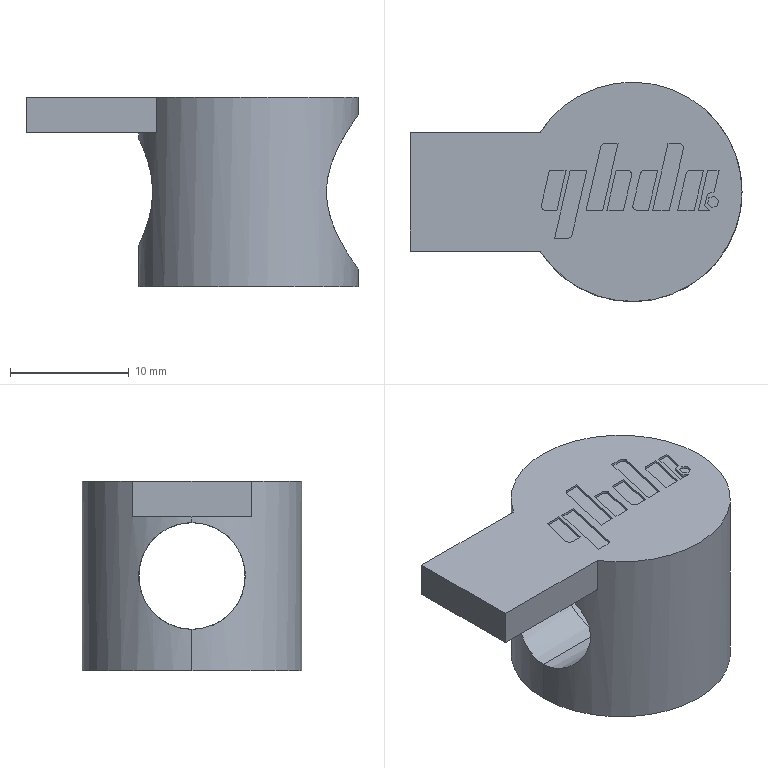Part | NX | features BREP 1 | 1 solid | 73 faces | box 28 x 18.5 x 16 mm | volume 2680 mm3 | plane 57 | cylinder 16 | commonest cylinder face diameters 0.702 x10 9 x2 13 x2 18.5 x2